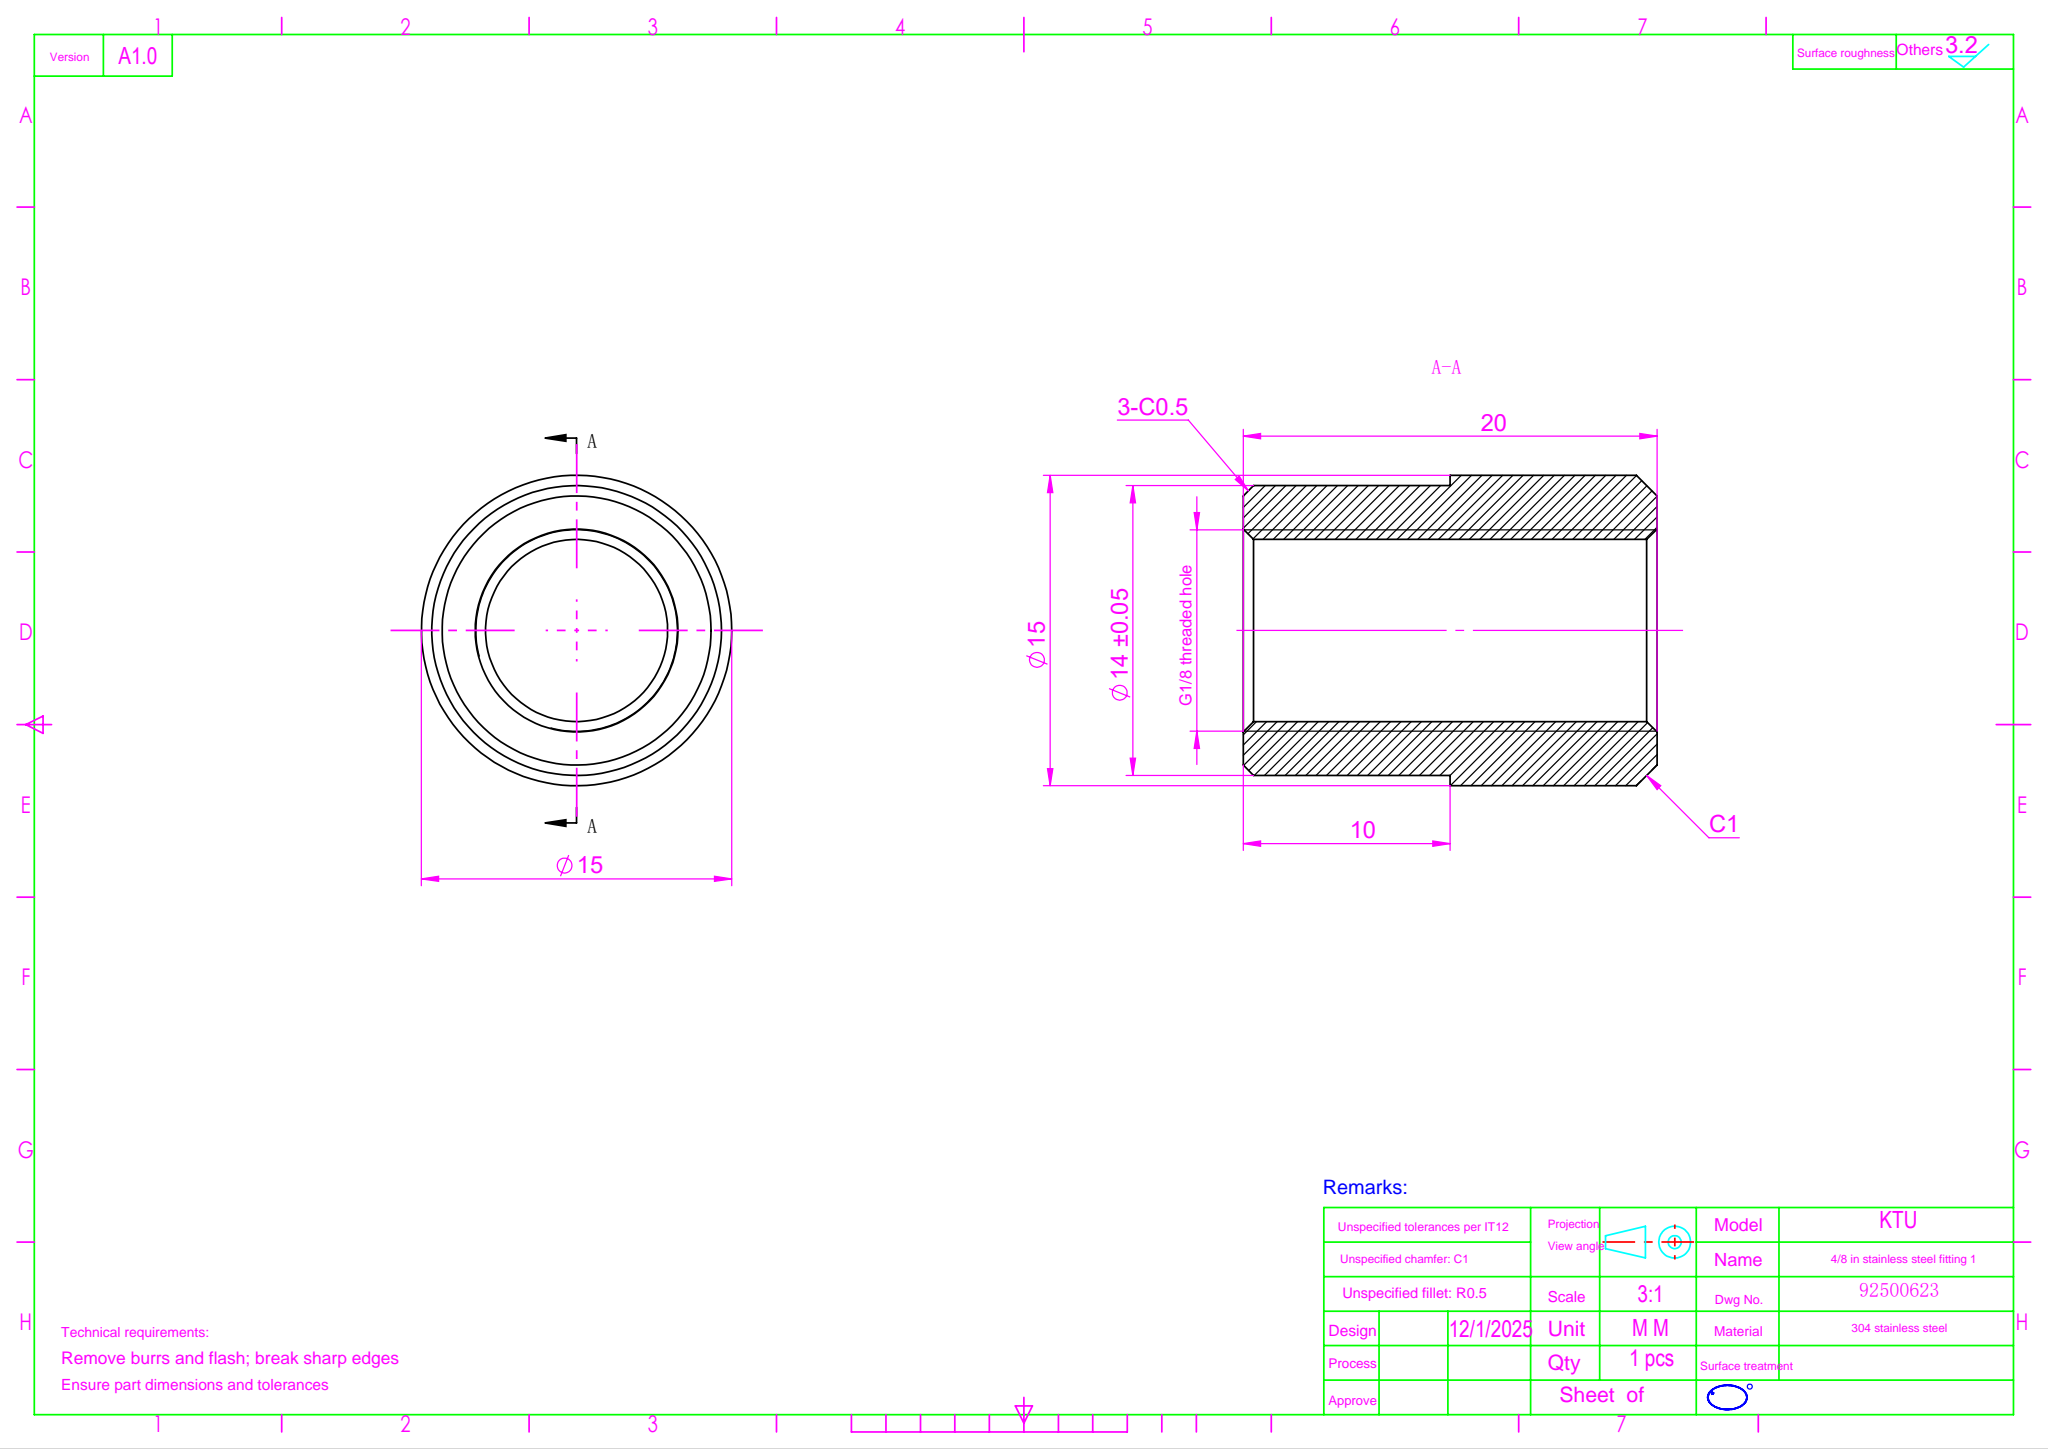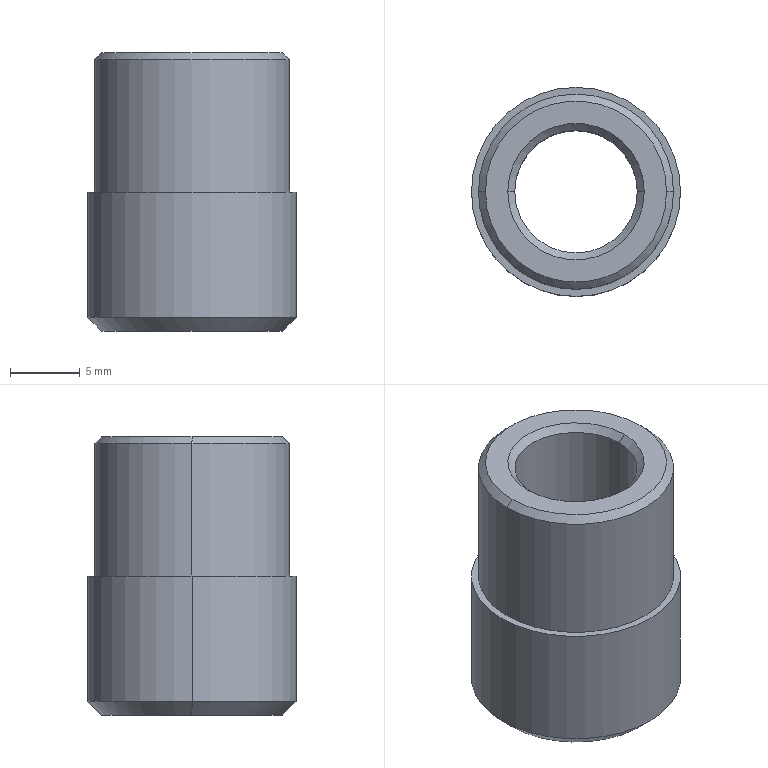Part | SolidWorks | features Chamfer 2, ICE 2, Extrusion 1, HoleWzd 1 | 1 solid | 17 faces | box 15 x 15 x 20 mm | volume 2055 mm3 | cone 8 | cylinder 6 | plane 3 | commonest cylinder face diameters 8.8 x2 14 x2 15 x2
STEP:
#1=CARTESIAN_POINT('',(6.5,0.,20.));
#2=VERTEX_POINT('',#1);
#3=CARTESIAN_POINT('',(-6.5,0.,20.));
#4=VERTEX_POINT('',#3);
#5=CARTESIAN_POINT('',(0.,0.,20.));
#6=DIRECTION('',(0.,0.,1.));
#7=DIRECTION('',(1.,0.,0.));
#8=AXIS2_PLACEMENT_3D('',#5,#6,#7);
#9=CIRCLE('',#8,6.5);
#10=EDGE_CURVE('',#2,#4,#9,.T.);
#11=ORIENTED_EDGE('',*,*,#10,.F.);
#12=CARTESIAN_POINT('',(7.,0.,19.5));
#13=VERTEX_POINT('',#12);
#14=CARTESIAN_POINT('',(6.5,0.,20.));
#15=DIRECTION('',(0.7071,0.,-0.7071));
#16=VECTOR('',#15,1000.);
#17=LINE('',#14,#16);
#18=EDGE_CURVE('',#2,#13,#17,.T.);
#19=ORIENTED_EDGE('',*,*,#18,.T.);
#20=CARTESIAN_POINT('',(-7.,0.,19.5));
#21=VERTEX_POINT('',#20);
#22=CARTESIAN_POINT('',(0.,0.,19.5));
#23=DIRECTION('',(0.,0.,-1.));
#24=DIRECTION('',(1.,0.,0.));
#25=AXIS2_PLACEMENT_3D('',#22,#23,#24);
#26=CIRCLE('',#25,7.);
#27=EDGE_CURVE('',#21,#13,#26,.T.);
#28=ORIENTED_EDGE('',*,*,#27,.F.);
#29=CARTESIAN_POINT('',(-6.5,0.,20.));
#30=DIRECTION('',(-0.7071,0.,-0.7071));
#31=VECTOR('',#30,1000.);
#32=LINE('',#29,#31);
#33=EDGE_CURVE('',#4,#21,#32,.T.);
#34=ORIENTED_EDGE('',*,*,#33,.F.);
#35=EDGE_LOOP('',(#11,#19,#28,#34));
#36=FACE_OUTER_BOUND('',#35,.T.);
#37=CARTESIAN_POINT('',(0.,0.,20.));
#38=DIRECTION('',(0.,0.,-1.));
#39=DIRECTION('',(-1.,0.,0.));
#40=AXIS2_PLACEMENT_3D('',#37,#38,#39);
#41=CONICAL_SURFACE('',#40,6.5,0.7854);
#42=ADVANCED_FACE('',(#36),#41,.T.);
#43=CARTESIAN_POINT('',(-4.4,0.,19.5));
#44=VERTEX_POINT('',#43);
#45=CARTESIAN_POINT('',(4.4,0.,19.5));
#46=VERTEX_POINT('',#45);
#47=CARTESIAN_POINT('',(0.,0.,19.5));
#48=DIRECTION('',(0.,0.,1.));
#49=DIRECTION('',(1.,0.,0.));
#50=AXIS2_PLACEMENT_3D('',#47,#48,#49);
#51=CIRCLE('',#50,4.4);
#52=EDGE_CURVE('',#44,#46,#51,.T.);
#53=ORIENTED_EDGE('',*,*,#52,.F.);
#54=CARTESIAN_POINT('',(-4.9,0.,20.));
#55=VERTEX_POINT('',#54);
#56=CARTESIAN_POINT('',(-4.4,0.,19.5));
#57=DIRECTION('',(-0.7071,0.,0.7071));
#58=VECTOR('',#57,1000.);
#59=LINE('',#56,#58);
#60=EDGE_CURVE('',#44,#55,#59,.T.);
#61=ORIENTED_EDGE('',*,*,#60,.T.);
#62=CARTESIAN_POINT('',(4.9,0.,20.));
#63=VERTEX_POINT('',#62);
#64=CARTESIAN_POINT('',(0.,0.,20.));
#65=DIRECTION('',(0.,0.,-1.));
#66=DIRECTION('',(1.,0.,0.));
#67=AXIS2_PLACEMENT_3D('',#64,#65,#66);
#68=CIRCLE('',#67,4.9);
#69=EDGE_CURVE('',#63,#55,#68,.T.);
#70=ORIENTED_EDGE('',*,*,#69,.F.);
#71=CARTESIAN_POINT('',(4.4,0.,19.5));
#72=DIRECTION('',(0.7071,0.,0.7071));
#73=VECTOR('',#72,1000.);
#74=LINE('',#71,#73);
#75=EDGE_CURVE('',#46,#63,#74,.T.);
#76=ORIENTED_EDGE('',*,*,#75,.F.);
#77=EDGE_LOOP('',(#53,#61,#70,#76));
#78=FACE_OUTER_BOUND('',#77,.T.);
#79=CARTESIAN_POINT('',(0.,0.,19.5));
#80=DIRECTION('',(0.,0.,1.));
#81=DIRECTION('',(1.,0.,0.));
#82=AXIS2_PLACEMENT_3D('',#79,#80,#81);
#83=CONICAL_SURFACE('',#82,4.4,0.7854);
#84=ADVANCED_FACE('',(#78),#83,.F.);
#85=CARTESIAN_POINT('',(4.4,0.,0.5));
#86=VERTEX_POINT('',#85);
#87=CARTESIAN_POINT('',(-4.4,0.,0.5));
#88=VERTEX_POINT('',#87);
#89=CARTESIAN_POINT('',(0.,0.,0.5));
#90=DIRECTION('',(0.,0.,-1.));
#91=DIRECTION('',(1.,0.,0.));
#92=AXIS2_PLACEMENT_3D('',#89,#90,#91);
#93=CIRCLE('',#92,4.4);
#94=EDGE_CURVE('',#86,#88,#93,.T.);
#95=ORIENTED_EDGE('',*,*,#94,.F.);
#96=CARTESIAN_POINT('',(4.9,0.,0.));
#97=VERTEX_POINT('',#96);
#98=CARTESIAN_POINT('',(4.9,0.,0.));
#99=DIRECTION('',(0.7071,0.,-0.7071));
#100=VECTOR('',#99,1000.);
#101=LINE('',#98,#100);
#102=EDGE_CURVE('',#86,#97,#101,.T.);
#103=ORIENTED_EDGE('',*,*,#102,.T.);
#104=CARTESIAN_POINT('',(-4.9,0.,0.));
#105=VERTEX_POINT('',#104);
#106=CARTESIAN_POINT('',(0.,0.,0.));
#107=DIRECTION('',(0.,0.,1.));
#108=DIRECTION('',(1.,0.,0.));
#109=AXIS2_PLACEMENT_3D('',#106,#107,#108);
#110=CIRCLE('',#109,4.9);
#111=EDGE_CURVE('',#105,#97,#110,.T.);
#112=ORIENTED_EDGE('',*,*,#111,.F.);
#113=CARTESIAN_POINT('',(-4.9,0.,0.));
#114=DIRECTION('',(-0.7071,0.,-0.7071));
#115=VECTOR('',#114,1000.);
#116=LINE('',#113,#115);
#117=EDGE_CURVE('',#88,#105,#116,.T.);
#118=ORIENTED_EDGE('',*,*,#117,.F.);
#119=EDGE_LOOP('',(#95,#103,#112,#118));
#120=FACE_OUTER_BOUND('',#119,.T.);
#121=CARTESIAN_POINT('',(0.,0.,0.));
#122=DIRECTION('',(0.,0.,-1.));
#123=DIRECTION('',(-1.,0.,0.));
#124=AXIS2_PLACEMENT_3D('',#121,#122,#123);
#125=CONICAL_SURFACE('',#124,4.9,0.7854);
#126=ADVANCED_FACE('',(#120),#125,.F.);
#127=CARTESIAN_POINT('',(-6.5,0.,0.));
#128=VERTEX_POINT('',#127);
#129=CARTESIAN_POINT('',(6.5,0.,0.));
#130=VERTEX_POINT('',#129);
#131=CARTESIAN_POINT('',(0.,0.,0.));
#132=DIRECTION('',(0.,0.,-1.));
#133=DIRECTION('',(1.,0.,0.));
#134=AXIS2_PLACEMENT_3D('',#131,#132,#133);
#135=CIRCLE('',#134,6.5);
#136=EDGE_CURVE('',#128,#130,#135,.T.);
#137=ORIENTED_EDGE('',*,*,#136,.F.);
#138=CARTESIAN_POINT('',(-7.5,0.,1.));
#139=VERTEX_POINT('',#138);
#140=CARTESIAN_POINT('',(-7.5,0.,1.));
#141=DIRECTION('',(-0.7071,0.,0.7071));
#142=VECTOR('',#141,1000.);
#143=LINE('',#140,#142);
#144=EDGE_CURVE('',#128,#139,#143,.T.);
#145=ORIENTED_EDGE('',*,*,#144,.T.);
#146=CARTESIAN_POINT('',(7.5,0.,1.));
#147=VERTEX_POINT('',#146);
#148=CARTESIAN_POINT('',(0.,0.,1.));
#149=DIRECTION('',(0.,0.,1.));
#150=DIRECTION('',(1.,0.,0.));
#151=AXIS2_PLACEMENT_3D('',#148,#149,#150);
#152=CIRCLE('',#151,7.5);
#153=EDGE_CURVE('',#147,#139,#152,.T.);
#154=ORIENTED_EDGE('',*,*,#153,.F.);
#155=CARTESIAN_POINT('',(7.5,0.,1.));
#156=DIRECTION('',(0.7071,0.,0.7071));
#157=VECTOR('',#156,1000.);
#158=LINE('',#155,#157);
#159=EDGE_CURVE('',#130,#147,#158,.T.);
#160=ORIENTED_EDGE('',*,*,#159,.F.);
#161=EDGE_LOOP('',(#137,#145,#154,#160));
#162=FACE_OUTER_BOUND('',#161,.T.);
#163=CARTESIAN_POINT('',(0.,0.,1.));
#164=DIRECTION('',(0.,0.,1.));
#165=DIRECTION('',(1.,0.,0.));
#166=AXIS2_PLACEMENT_3D('',#163,#164,#165);
#167=CONICAL_SURFACE('',#166,7.5,0.7854);
#168=ADVANCED_FACE('',(#162),#167,.T.);
#169=ORIENTED_EDGE('',*,*,#94,.T.);
#170=CARTESIAN_POINT('',(-4.4,0.,20.));
#171=DIRECTION('',(0.,0.,1.));
#172=VECTOR('',#171,1000.);
#173=LINE('',#170,#172);
#174=EDGE_CURVE('',#88,#44,#173,.T.);
#175=ORIENTED_EDGE('',*,*,#174,.T.);
#176=ORIENTED_EDGE('',*,*,#52,.T.);
#177=CARTESIAN_POINT('',(4.4,0.,20.));
#178=DIRECTION('',(0.,0.,1.));
#179=VECTOR('',#178,1000.);
#180=LINE('',#177,#179);
#181=EDGE_CURVE('',#86,#46,#180,.T.);
#182=ORIENTED_EDGE('',*,*,#181,.F.);
#183=EDGE_LOOP('',(#169,#175,#176,#182));
#184=FACE_OUTER_BOUND('',#183,.T.);
#185=CARTESIAN_POINT('',(0.,0.,20.));
#186=DIRECTION('',(0.,0.,1.));
#187=DIRECTION('',(1.,0.,0.));
#188=AXIS2_PLACEMENT_3D('',#185,#186,#187);
#189=CYLINDRICAL_SURFACE('',#188,4.4);
#190=ADVANCED_FACE('',(#184),#189,.F.);
#191=CARTESIAN_POINT('',(7.,0.,10.));
#192=VERTEX_POINT('',#191);
#193=CARTESIAN_POINT('',(-7.,0.,10.));
#194=VERTEX_POINT('',#193);
#195=CARTESIAN_POINT('',(0.,0.,10.));
#196=DIRECTION('',(0.,0.,1.));
#197=DIRECTION('',(1.,0.,0.));
#198=AXIS2_PLACEMENT_3D('',#195,#196,#197);
#199=CIRCLE('',#198,7.);
#200=EDGE_CURVE('',#192,#194,#199,.T.);
#201=ORIENTED_EDGE('',*,*,#200,.T.);
#202=CARTESIAN_POINT('',(-7.,0.,10.));
#203=DIRECTION('',(0.,0.,1.));
#204=VECTOR('',#203,1000.);
#205=LINE('',#202,#204);
#206=EDGE_CURVE('',#194,#21,#205,.T.);
#207=ORIENTED_EDGE('',*,*,#206,.T.);
#208=ORIENTED_EDGE('',*,*,#27,.T.);
#209=CARTESIAN_POINT('',(7.,0.,10.));
#210=DIRECTION('',(0.,0.,1.));
#211=VECTOR('',#210,1000.);
#212=LINE('',#209,#211);
#213=EDGE_CURVE('',#192,#13,#212,.T.);
#214=ORIENTED_EDGE('',*,*,#213,.F.);
#215=EDGE_LOOP('',(#201,#207,#208,#214));
#216=FACE_OUTER_BOUND('',#215,.T.);
#217=CARTESIAN_POINT('',(0.,0.,10.));
#218=DIRECTION('',(0.,0.,1.));
#219=DIRECTION('',(1.,0.,0.));
#220=AXIS2_PLACEMENT_3D('',#217,#218,#219);
#221=CYLINDRICAL_SURFACE('',#220,7.);
#222=ADVANCED_FACE('',(#216),#221,.T.);
#223=CARTESIAN_POINT('',(7.5,0.,10.));
#224=VERTEX_POINT('',#223);
#225=CARTESIAN_POINT('',(-7.5,0.,10.));
#226=VERTEX_POINT('',#225);
#227=CARTESIAN_POINT('',(0.,0.,10.));
#228=DIRECTION('',(0.,0.,1.));
#229=DIRECTION('',(1.,0.,0.));
#230=AXIS2_PLACEMENT_3D('',#227,#228,#229);
#231=CIRCLE('',#230,7.5);
#232=EDGE_CURVE('',#224,#226,#231,.T.);
#233=ORIENTED_EDGE('',*,*,#232,.F.);
#234=CARTESIAN_POINT('',(7.5,0.,20.));
#235=DIRECTION('',(0.,0.,-1.));
#236=VECTOR('',#235,1000.);
#237=LINE('',#234,#236);
#238=EDGE_CURVE('',#224,#147,#237,.T.);
#239=ORIENTED_EDGE('',*,*,#238,.T.);
#240=ORIENTED_EDGE('',*,*,#153,.T.);
#241=CARTESIAN_POINT('',(-7.5,0.,20.));
#242=DIRECTION('',(0.,0.,-1.));
#243=VECTOR('',#242,1000.);
#244=LINE('',#241,#243);
#245=EDGE_CURVE('',#226,#139,#244,.T.);
#246=ORIENTED_EDGE('',*,*,#245,.F.);
#247=EDGE_LOOP('',(#233,#239,#240,#246));
#248=FACE_OUTER_BOUND('',#247,.T.);
#249=CARTESIAN_POINT('',(0.,0.,20.));
#250=DIRECTION('',(0.,0.,-1.));
#251=DIRECTION('',(-1.,0.,0.));
#252=AXIS2_PLACEMENT_3D('',#249,#250,#251);
#253=CYLINDRICAL_SURFACE('',#252,7.5);
#254=ADVANCED_FACE('',(#248),#253,.T.);
#255=ORIENTED_EDGE('',*,*,#238,.F.);
#256=CARTESIAN_POINT('',(0.,0.,10.));
#257=DIRECTION('',(0.,0.,1.));
#258=DIRECTION('',(1.,0.,0.));
#259=AXIS2_PLACEMENT_3D('',#256,#257,#258);
#260=CIRCLE('',#259,7.5);
#261=EDGE_CURVE('',#226,#224,#260,.T.);
#262=ORIENTED_EDGE('',*,*,#261,.F.);
#263=ORIENTED_EDGE('',*,*,#245,.T.);
#264=CARTESIAN_POINT('',(0.,0.,1.));
#265=DIRECTION('',(0.,0.,1.));
#266=DIRECTION('',(1.,0.,0.));
#267=AXIS2_PLACEMENT_3D('',#264,#265,#266);
#268=CIRCLE('',#267,7.5);
#269=EDGE_CURVE('',#139,#147,#268,.T.);
#270=ORIENTED_EDGE('',*,*,#269,.T.);
#271=EDGE_LOOP('',(#255,#262,#263,#270));
#272=FACE_OUTER_BOUND('',#271,.T.);
#273=CARTESIAN_POINT('',(0.,0.,20.));
#274=DIRECTION('',(0.,0.,-1.));
#275=DIRECTION('',(-1.,0.,0.));
#276=AXIS2_PLACEMENT_3D('',#273,#274,#275);
#277=CYLINDRICAL_SURFACE('',#276,7.5);
#278=ADVANCED_FACE('',(#272),#277,.T.);
#279=ORIENTED_EDGE('',*,*,#111,.T.);
#280=CARTESIAN_POINT('',(0.,0.,0.));
#281=DIRECTION('',(0.,0.,1.));
#282=DIRECTION('',(1.,0.,0.));
#283=AXIS2_PLACEMENT_3D('',#280,#281,#282);
#284=CIRCLE('',#283,4.9);
#285=EDGE_CURVE('',#97,#105,#284,.T.);
#286=ORIENTED_EDGE('',*,*,#285,.T.);
#287=EDGE_LOOP('',(#279,#286));
#288=FACE_BOUND('',#287,.T.);
#289=CARTESIAN_POINT('',(0.,0.,0.));
#290=DIRECTION('',(0.,0.,-1.));
#291=DIRECTION('',(1.,0.,0.));
#292=AXIS2_PLACEMENT_3D('',#289,#290,#291);
#293=CIRCLE('',#292,6.5);
#294=EDGE_CURVE('',#130,#128,#293,.T.);
#295=ORIENTED_EDGE('',*,*,#294,.T.);
#296=ORIENTED_EDGE('',*,*,#136,.T.);
#297=EDGE_LOOP('',(#295,#296));
#298=FACE_OUTER_BOUND('',#297,.T.);
#299=CARTESIAN_POINT('',(0.,0.,0.));
#300=DIRECTION('',(0.,0.,1.));
#301=DIRECTION('',(1.,0.,0.));
#302=AXIS2_PLACEMENT_3D('',#299,#300,#301);
#303=PLANE('',#302);
#304=ADVANCED_FACE('',(#288,#298),#303,.F.);
#305=ORIENTED_EDGE('',*,*,#200,.F.);
#306=CARTESIAN_POINT('',(0.,0.,10.));
#307=DIRECTION('',(0.,0.,1.));
#308=DIRECTION('',(1.,0.,0.));
#309=AXIS2_PLACEMENT_3D('',#306,#307,#308);
#310=CIRCLE('',#309,7.);
#311=EDGE_CURVE('',#194,#192,#310,.T.);
#312=ORIENTED_EDGE('',*,*,#311,.F.);
#313=EDGE_LOOP('',(#305,#312));
#314=FACE_BOUND('',#313,.T.);
#315=ORIENTED_EDGE('',*,*,#261,.T.);
#316=ORIENTED_EDGE('',*,*,#232,.T.);
#317=EDGE_LOOP('',(#315,#316));
#318=FACE_OUTER_BOUND('',#317,.T.);
#319=CARTESIAN_POINT('',(0.,0.,10.));
#320=DIRECTION('',(0.,0.,1.));
#321=DIRECTION('',(1.,0.,0.));
#322=AXIS2_PLACEMENT_3D('',#319,#320,#321);
#323=PLANE('',#322);
#324=ADVANCED_FACE('',(#314,#318),#323,.T.);
#325=ORIENTED_EDGE('',*,*,#206,.F.);
#326=ORIENTED_EDGE('',*,*,#311,.T.);
#327=ORIENTED_EDGE('',*,*,#213,.T.);
#328=CARTESIAN_POINT('',(0.,0.,19.5));
#329=DIRECTION('',(0.,0.,-1.));
#330=DIRECTION('',(1.,0.,0.));
#331=AXIS2_PLACEMENT_3D('',#328,#329,#330);
#332=CIRCLE('',#331,7.);
#333=EDGE_CURVE('',#13,#21,#332,.T.);
#334=ORIENTED_EDGE('',*,*,#333,.T.);
#335=EDGE_LOOP('',(#325,#326,#327,#334));
#336=FACE_OUTER_BOUND('',#335,.T.);
#337=CARTESIAN_POINT('',(0.,0.,10.));
#338=DIRECTION('',(0.,0.,1.));
#339=DIRECTION('',(1.,0.,0.));
#340=AXIS2_PLACEMENT_3D('',#337,#338,#339);
#341=CYLINDRICAL_SURFACE('',#340,7.);
#342=ADVANCED_FACE('',(#336),#341,.T.);
#343=ORIENTED_EDGE('',*,*,#69,.T.);
#344=CARTESIAN_POINT('',(0.,0.,20.));
#345=DIRECTION('',(0.,0.,-1.));
#346=DIRECTION('',(1.,0.,0.));
#347=AXIS2_PLACEMENT_3D('',#344,#345,#346);
#348=CIRCLE('',#347,4.9);
#349=EDGE_CURVE('',#55,#63,#348,.T.);
#350=ORIENTED_EDGE('',*,*,#349,.T.);
#351=EDGE_LOOP('',(#343,#350));
#352=FACE_BOUND('',#351,.T.);
#353=CARTESIAN_POINT('',(0.,0.,20.));
#354=DIRECTION('',(0.,0.,1.));
#355=DIRECTION('',(1.,0.,0.));
#356=AXIS2_PLACEMENT_3D('',#353,#354,#355);
#357=CIRCLE('',#356,6.5);
#358=EDGE_CURVE('',#4,#2,#357,.T.);
#359=ORIENTED_EDGE('',*,*,#358,.T.);
#360=ORIENTED_EDGE('',*,*,#10,.T.);
#361=EDGE_LOOP('',(#359,#360));
#362=FACE_OUTER_BOUND('',#361,.T.);
#363=CARTESIAN_POINT('',(0.,0.,20.));
#364=DIRECTION('',(0.,0.,1.));
#365=DIRECTION('',(1.,0.,0.));
#366=AXIS2_PLACEMENT_3D('',#363,#364,#365);
#367=PLANE('',#366);
#368=ADVANCED_FACE('',(#352,#362),#367,.T.);
#369=ORIENTED_EDGE('',*,*,#174,.F.);
#370=CARTESIAN_POINT('',(0.,0.,0.5));
#371=DIRECTION('',(0.,0.,-1.));
#372=DIRECTION('',(1.,0.,0.));
#373=AXIS2_PLACEMENT_3D('',#370,#371,#372);
#374=CIRCLE('',#373,4.4);
#375=EDGE_CURVE('',#88,#86,#374,.T.);
#376=ORIENTED_EDGE('',*,*,#375,.T.);
#377=ORIENTED_EDGE('',*,*,#181,.T.);
#378=CARTESIAN_POINT('',(0.,0.,19.5));
#379=DIRECTION('',(0.,0.,1.));
#380=DIRECTION('',(1.,0.,0.));
#381=AXIS2_PLACEMENT_3D('',#378,#379,#380);
#382=CIRCLE('',#381,4.4);
#383=EDGE_CURVE('',#46,#44,#382,.T.);
#384=ORIENTED_EDGE('',*,*,#383,.T.);
#385=EDGE_LOOP('',(#369,#376,#377,#384));
#386=FACE_OUTER_BOUND('',#385,.T.);
#387=CARTESIAN_POINT('',(0.,0.,20.));
#388=DIRECTION('',(0.,0.,1.));
#389=DIRECTION('',(1.,0.,0.));
#390=AXIS2_PLACEMENT_3D('',#387,#388,#389);
#391=CYLINDRICAL_SURFACE('',#390,4.4);
#392=ADVANCED_FACE('',(#386),#391,.F.);
#393=ORIENTED_EDGE('',*,*,#144,.F.);
#394=ORIENTED_EDGE('',*,*,#294,.F.);
#395=ORIENTED_EDGE('',*,*,#159,.T.);
#396=ORIENTED_EDGE('',*,*,#269,.F.);
#397=EDGE_LOOP('',(#393,#394,#395,#396));
#398=FACE_OUTER_BOUND('',#397,.T.);
#399=CARTESIAN_POINT('',(0.,0.,1.));
#400=DIRECTION('',(0.,0.,1.));
#401=DIRECTION('',(1.,0.,0.));
#402=AXIS2_PLACEMENT_3D('',#399,#400,#401);
#403=CONICAL_SURFACE('',#402,7.5,0.7854);
#404=ADVANCED_FACE('',(#398),#403,.T.);
#405=ORIENTED_EDGE('',*,*,#102,.F.);
#406=ORIENTED_EDGE('',*,*,#375,.F.);
#407=ORIENTED_EDGE('',*,*,#117,.T.);
#408=ORIENTED_EDGE('',*,*,#285,.F.);
#409=EDGE_LOOP('',(#405,#406,#407,#408));
#410=FACE_OUTER_BOUND('',#409,.T.);
#411=CARTESIAN_POINT('',(0.,0.,0.));
#412=DIRECTION('',(0.,0.,-1.));
#413=DIRECTION('',(-1.,0.,0.));
#414=AXIS2_PLACEMENT_3D('',#411,#412,#413);
#415=CONICAL_SURFACE('',#414,4.9,0.7854);
#416=ADVANCED_FACE('',(#410),#415,.F.);
#417=ORIENTED_EDGE('',*,*,#60,.F.);
#418=ORIENTED_EDGE('',*,*,#383,.F.);
#419=ORIENTED_EDGE('',*,*,#75,.T.);
#420=ORIENTED_EDGE('',*,*,#349,.F.);
#421=EDGE_LOOP('',(#417,#418,#419,#420));
#422=FACE_OUTER_BOUND('',#421,.T.);
#423=CARTESIAN_POINT('',(0.,0.,19.5));
#424=DIRECTION('',(0.,0.,1.));
#425=DIRECTION('',(1.,0.,0.));
#426=AXIS2_PLACEMENT_3D('',#423,#424,#425);
#427=CONICAL_SURFACE('',#426,4.4,0.7854);
#428=ADVANCED_FACE('',(#422),#427,.F.);
#429=ORIENTED_EDGE('',*,*,#18,.F.);
#430=ORIENTED_EDGE('',*,*,#358,.F.);
#431=ORIENTED_EDGE('',*,*,#33,.T.);
#432=ORIENTED_EDGE('',*,*,#333,.F.);
#433=EDGE_LOOP('',(#429,#430,#431,#432));
#434=FACE_OUTER_BOUND('',#433,.T.);
#435=CARTESIAN_POINT('',(0.,0.,20.));
#436=DIRECTION('',(0.,0.,-1.));
#437=DIRECTION('',(-1.,0.,0.));
#438=AXIS2_PLACEMENT_3D('',#435,#436,#437);
#439=CONICAL_SURFACE('',#438,6.5,0.7854);
#440=ADVANCED_FACE('',(#434),#439,.T.);
#441=CLOSED_SHELL('',(#42,#84,#126,#168,#190,#222,#254,#278,#304,#324,#342,#368,#392,#404,#416,#428,#440));
#442=MANIFOLD_SOLID_BREP('',#441);
#443=CARTESIAN_POINT('',(0.,0.,0.));
#444=DIRECTION('',(0.,0.,1.));
#445=DIRECTION('',(1.,0.,0.));
#446=AXIS2_PLACEMENT_3D('',#443,#444,#445);
#447=(LENGTH_UNIT()NAMED_UNIT(*)SI_UNIT(.MILLI.,.METRE.));
#448=UNCERTAINTY_MEASURE_WITH_UNIT(LENGTH_MEASURE(0.00001),#447,'','');
#449=(NAMED_UNIT(*)PLANE_ANGLE_UNIT()SI_UNIT($,.RADIAN.));
#450=(NAMED_UNIT(*)SI_UNIT($,.STERADIAN.)SOLID_ANGLE_UNIT());
#451=(GEOMETRIC_REPRESENTATION_CONTEXT(3)GLOBAL_UNCERTAINTY_ASSIGNED_CONTEXT((#448))GLOBAL_UNIT_ASSIGNED_CONTEXT((#447,#449,#450))REPRESENTATION_CONTEXT('',''));
#452=ADVANCED_BREP_SHAPE_REPRESENTATION('',(#442,#446),#451);